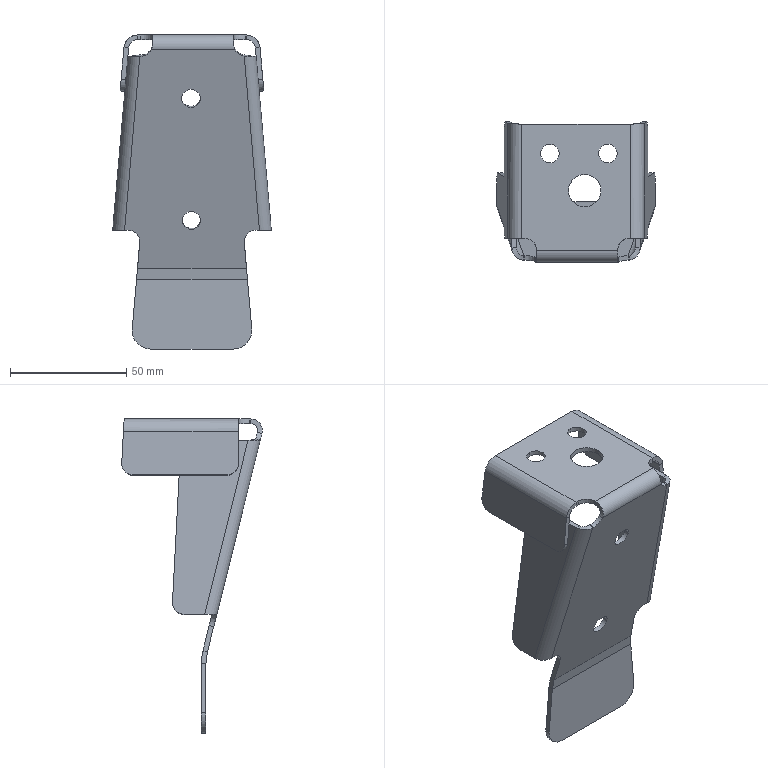Part | 1 solid | 90 faces | box 68.386 x 60.531 x 135.375 mm | volume 31573 mm3 | spline 32 | plane 28 | cylinder 24 | other 6 | commonest cylinder face diameters 8 x10 6 x3 10 x3 12 x2 14 x2 16 x2